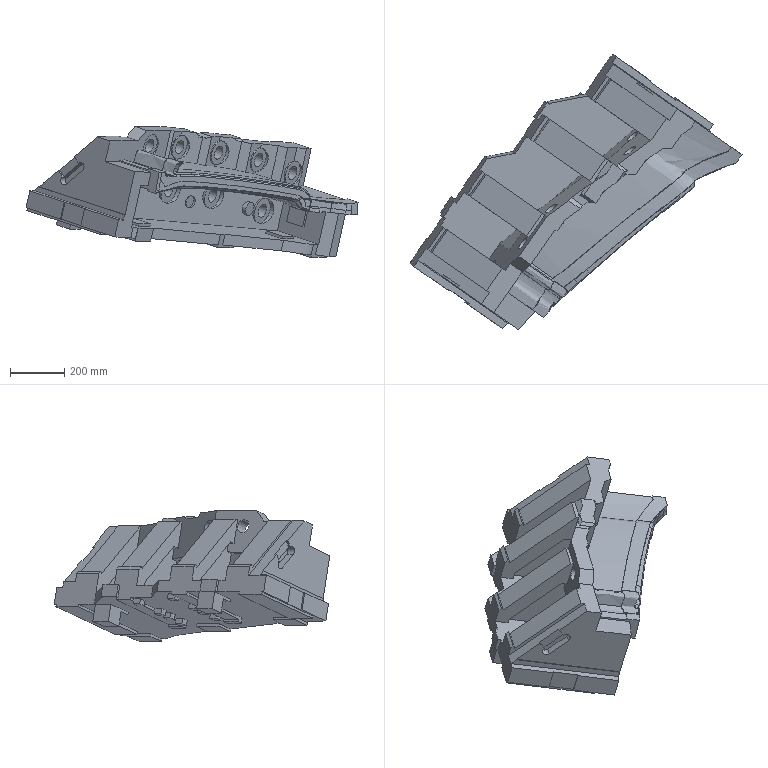Part | NX | features solid 2 | 1 solid | 492 faces | box 1222 x 1015 x 481.579 mm | volume 72976576 mm3 | plane 287 | spline 172 | cylinder 33 | commonest cylinder face diameters 50 x9 90 x9 96 x7 32 x4 45.4 x3 49.4 x1